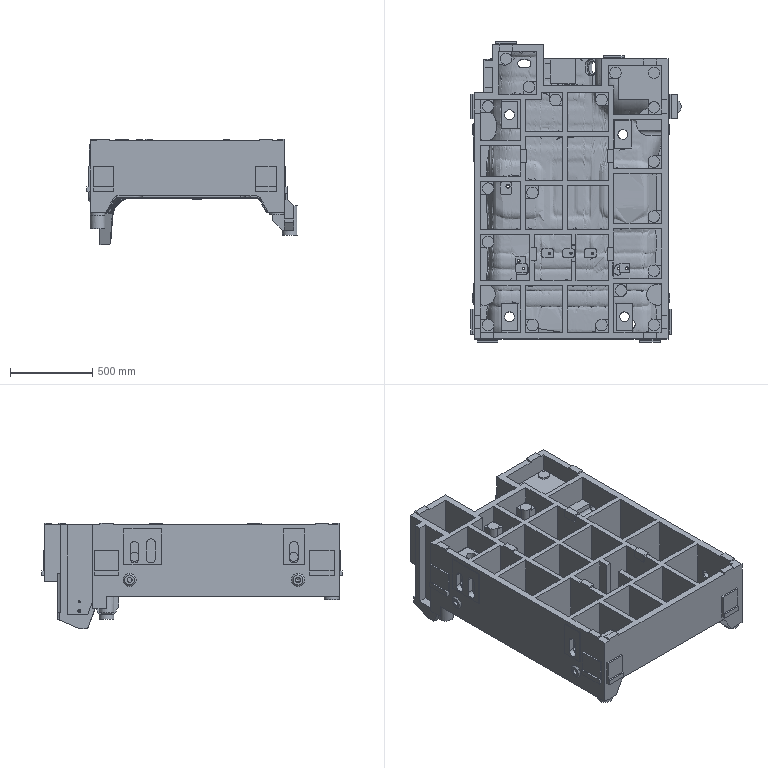Part | NX | features solid 2 | 1 solid | 2801 faces | box 1280 x 1830 x 643.1 mm | volume 297065976 mm3 | spline 1039 | plane 913 | cylinder 767 | sphere 35 | torus 26 | cone 21 | commonest cylinder face diameters 16 x156 20 x67 10 x57 12 x29 30 x26 100 x24